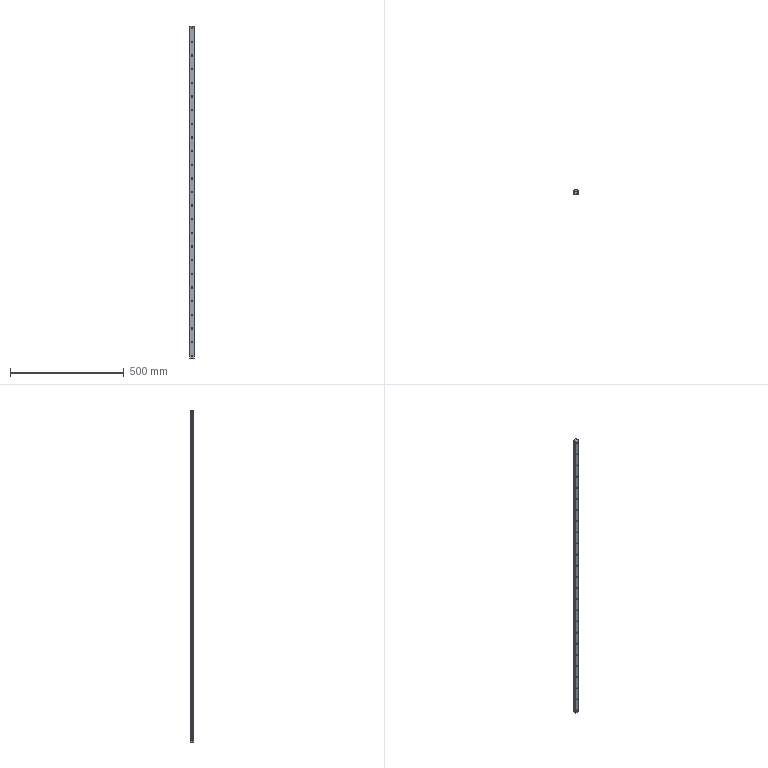Part | NX | 1 solid | 119 faces | box 20 x 17.5 x 1460 mm | volume 416869 mm3 | cylinder 72 | plane 47 | commonest cylinder face diameters 6 x25 10 x25 1 x12 2 x6 4.06 x4